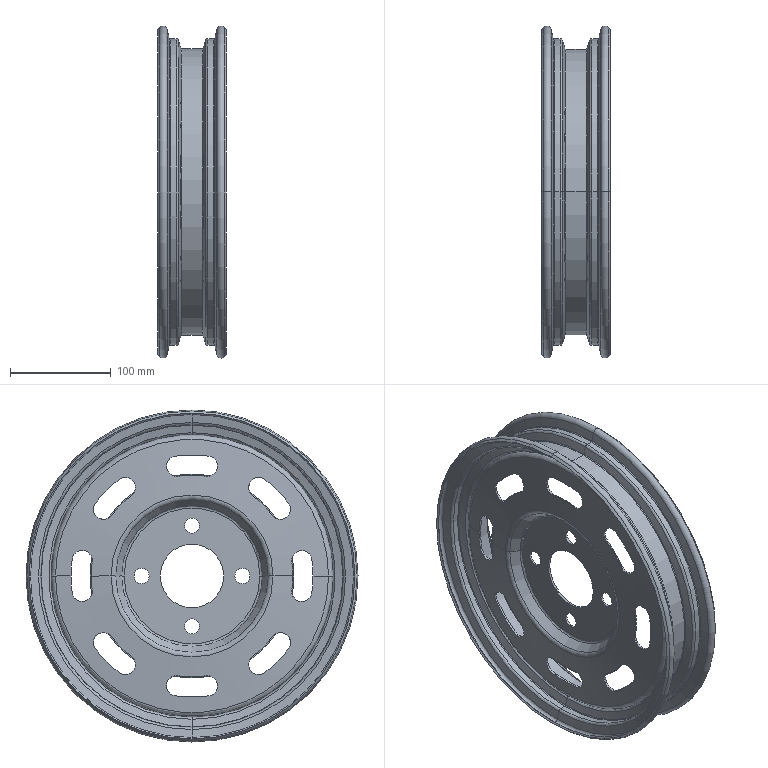Part | SolidWorks | 2 solids | 159 faces | box 67.896 x 329.277 x 329.277 mm | volume 312051 mm3 | cylinder 68 | torus 44 | cone 36 | plane 11 | commonest cylinder face diameters 20 x24 200 x9 240 x9 15 x8 300.503 x4 304 x4